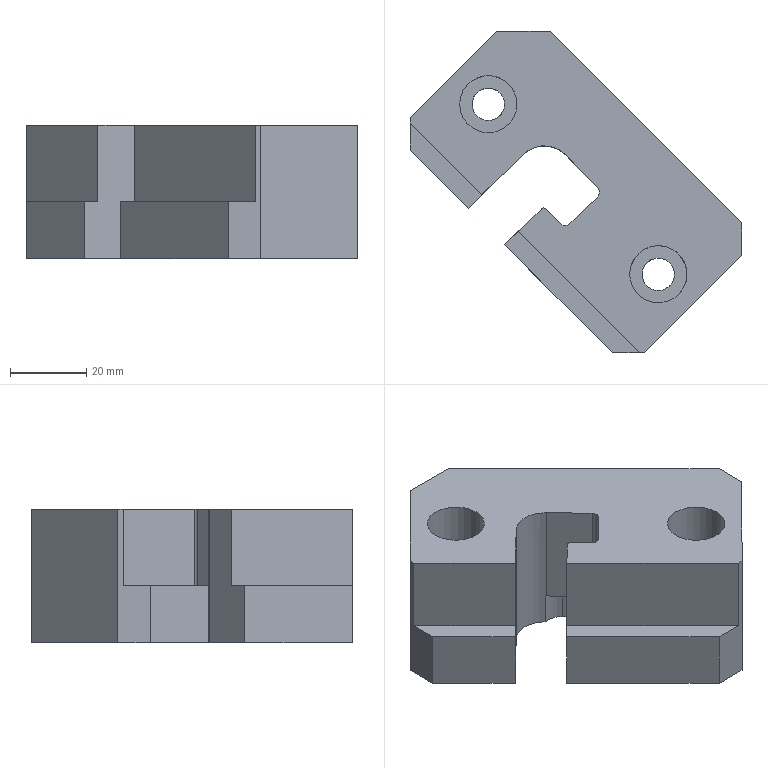Part | STEP file | gslz 2016.10.28-13_id542_x_t | 1 solid | 34 faces | box 86.974 x 84.146 x 35 mm | volume 110170 mm3 | plane 24 | cylinder 10 | commonest cylinder face diameters 3.5 x2 8.5 x2 11 x2 15 x2 2 x1 15.5 x1